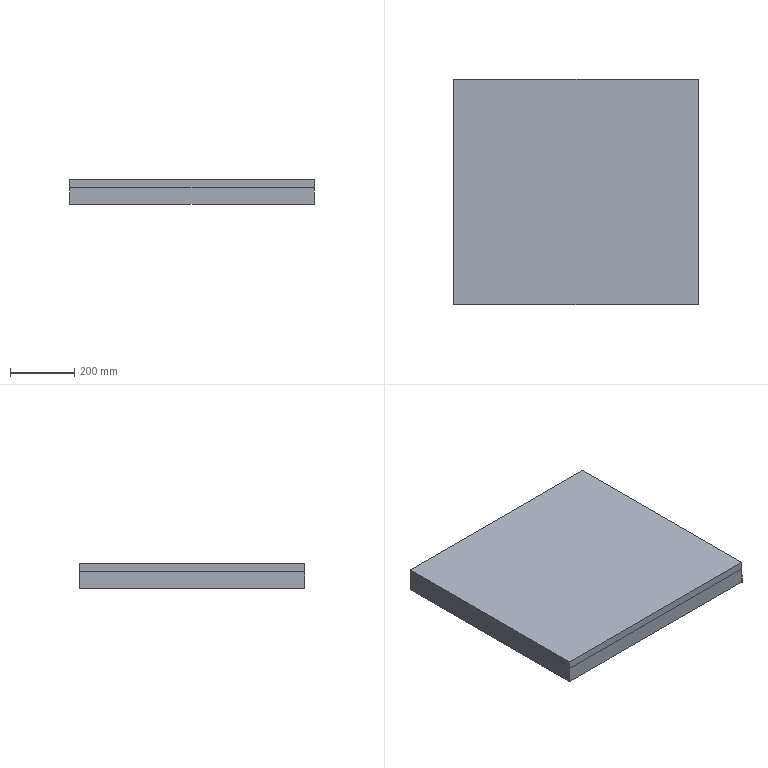Part | SolidWorks | features ICE 1, WeldMemberFeat 1, WeldmentFeature 1 | 5 solids | 74 faces | box 758 x 700 x 75 mm | volume 15208825 mm3 | plane 58 | cylinder 16 | commonest cylinder face diameters 7 x8 14 x8